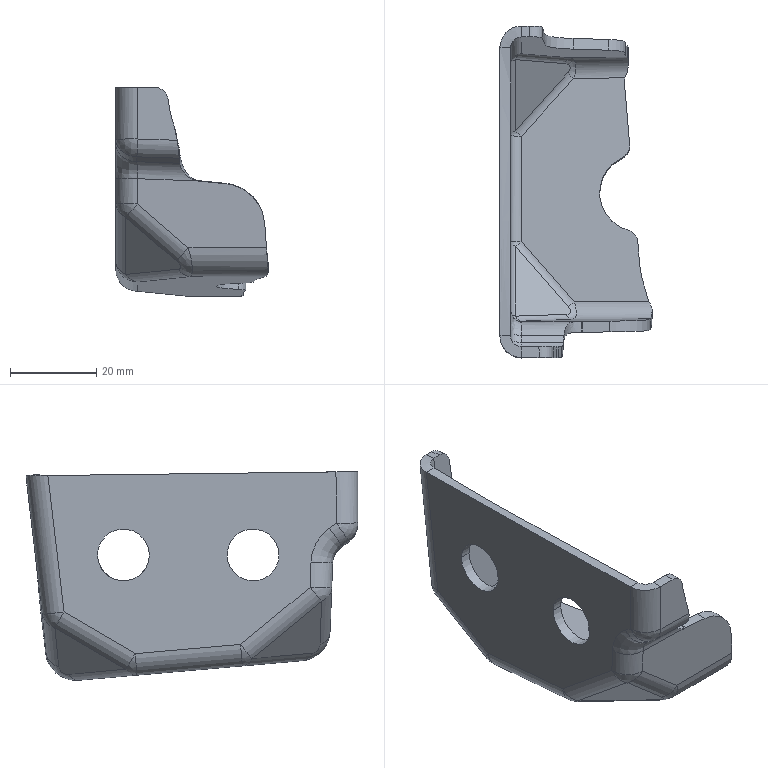Part | 1 solid | 110 faces | box 35.248 x 76.828 x 48.325 mm | volume 14168 mm3 | spline 43 | cylinder 39 | plane 18 | sphere 10 | commonest cylinder face diameters 10 x14 5 x12 12 x4 6 x2 9 x2 14 x2